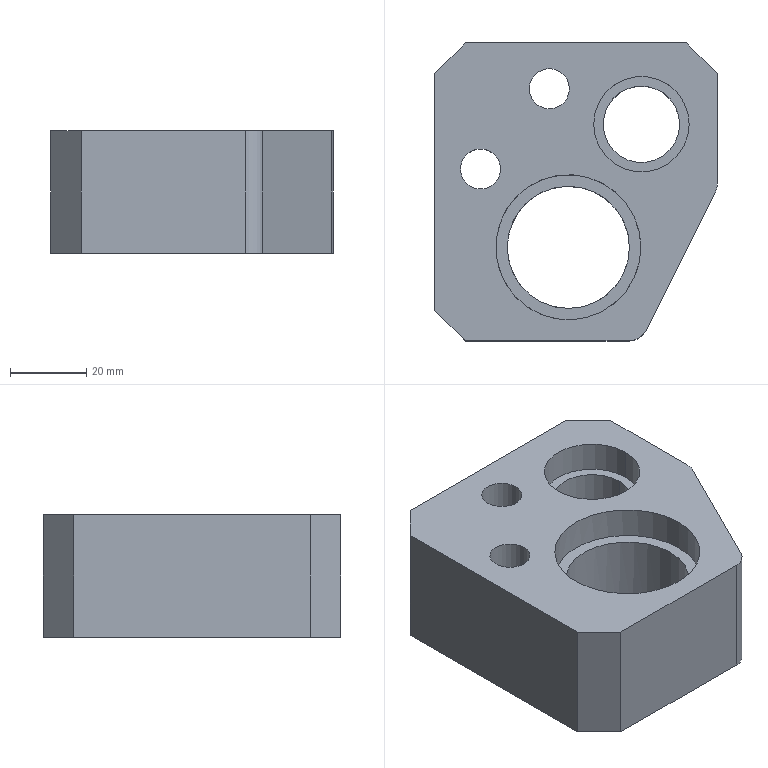Part | STEP file | lll_id3666_x_t | 1 solid | 26 faces | box 74 x 78 x 32 mm | volume 118554 mm3 | plane 14 | cylinder 12 | commonest cylinder face diameters 10 x2 10.5 x2 17 x2 20 x2 25 x2 32 x1
STEP:
#1=CARTESIAN_POINT('',(3317.117,63.788,77.5));
#2=VERTEX_POINT('',#1);
#3=CARTESIAN_POINT('',(3322.367,63.788,77.5));
#4=DIRECTION('',(0.,0.,1.));
#5=DIRECTION('',(-1.,0.,0.));
#6=AXIS2_PLACEMENT_3D('',#3,#4,#5);
#7=CIRCLE('',#6,5.25);
#8=EDGE_CURVE('',#2,#2,#7,.T.);
#9=ORIENTED_EDGE('',*,*,#8,.T.);
#10=EDGE_LOOP('',(#9));
#11=FACE_BOUND('',#10,.T.);
#12=CARTESIAN_POINT('',(3313.867,63.788,77.5));
#13=VERTEX_POINT('',#12);
#14=CARTESIAN_POINT('',(3322.367,63.788,77.5));
#15=DIRECTION('',(0.,0.,1.));
#16=DIRECTION('',(-1.,0.,0.));
#17=AXIS2_PLACEMENT_3D('',#14,#15,#16);
#18=CIRCLE('',#17,8.5);
#19=EDGE_CURVE('',#13,#13,#18,.T.);
#20=ORIENTED_EDGE('',*,*,#19,.F.);
#21=EDGE_LOOP('',(#20));
#22=FACE_BOUND('',#21,.T.);
#23=CARTESIAN_POINT('',(3322.367,63.788,77.5));
#24=DIRECTION('',(0.,0.,1.));
#25=DIRECTION('',(-1.,0.,0.));
#26=AXIS2_PLACEMENT_3D('',#23,#24,#25);
#27=PLANE('',#26);
#28=ADVANCED_FACE('',(#11,#22),#27,.F.);
#29=CARTESIAN_POINT('',(3326.367,43.288,84.3));
#30=VERTEX_POINT('',#29);
#31=CARTESIAN_POINT('',(3345.367,43.288,84.3));
#32=DIRECTION('',(0.,0.,1.));
#33=DIRECTION('',(-1.,0.,0.));
#34=AXIS2_PLACEMENT_3D('',#31,#32,#33);
#35=CIRCLE('',#34,19.);
#36=EDGE_CURVE('',#30,#30,#35,.T.);
#37=ORIENTED_EDGE('',*,*,#36,.T.);
#38=EDGE_LOOP('',(#37));
#39=FACE_BOUND('',#38,.T.);
#40=CARTESIAN_POINT('',(3329.367,43.288,84.3));
#41=VERTEX_POINT('',#40);
#42=CARTESIAN_POINT('',(3345.367,43.288,84.3));
#43=DIRECTION('',(0.,0.,1.));
#44=DIRECTION('',(-1.,0.,0.));
#45=AXIS2_PLACEMENT_3D('',#42,#43,#44);
#46=CIRCLE('',#45,16.);
#47=EDGE_CURVE('',#41,#41,#46,.T.);
#48=ORIENTED_EDGE('',*,*,#47,.F.);
#49=EDGE_LOOP('',(#48));
#50=FACE_BOUND('',#49,.T.);
#51=CARTESIAN_POINT('',(3345.367,52.038,84.3));
#52=DIRECTION('',(0.,0.,-1.));
#53=DIRECTION('',(0.,1.,0.));
#54=AXIS2_PLACEMENT_3D('',#51,#52,#53);
#55=PLANE('',#54);
#56=ADVANCED_FACE('',(#39,#50),#55,.F.);
#57=CARTESIAN_POINT('',(3352.,75.5,84.5));
#58=VERTEX_POINT('',#57);
#59=CARTESIAN_POINT('',(3377.,75.5,84.5));
#60=VERTEX_POINT('',#59);
#61=CARTESIAN_POINT('',(3364.5,75.5,84.5));
#62=DIRECTION('',(0.,0.,-1.));
#63=DIRECTION('',(1.,0.,0.));
#64=AXIS2_PLACEMENT_3D('',#61,#62,#63);
#65=CIRCLE('',#64,12.5);
#66=EDGE_CURVE('',#58,#60,#65,.T.);
#67=ORIENTED_EDGE('',*,*,#66,.F.);
#68=CARTESIAN_POINT('',(3364.5,75.5,84.5));
#69=DIRECTION('',(0.,0.,-1.));
#70=DIRECTION('',(1.,0.,0.));
#71=AXIS2_PLACEMENT_3D('',#68,#69,#70);
#72=CIRCLE('',#71,12.5);
#73=EDGE_CURVE('',#60,#58,#72,.T.);
#74=ORIENTED_EDGE('',*,*,#73,.F.);
#75=EDGE_LOOP('',(#67,#74));
#76=FACE_BOUND('',#75,.T.);
#77=CARTESIAN_POINT('',(3354.5,75.5,84.5));
#78=VERTEX_POINT('',#77);
#79=CARTESIAN_POINT('',(3374.5,75.5,84.5));
#80=VERTEX_POINT('',#79);
#81=CARTESIAN_POINT('',(3364.5,75.5,84.5));
#82=DIRECTION('',(0.,0.,-1.));
#83=DIRECTION('',(1.,0.,0.));
#84=AXIS2_PLACEMENT_3D('',#81,#82,#83);
#85=CIRCLE('',#84,10.);
#86=EDGE_CURVE('',#78,#80,#85,.T.);
#87=ORIENTED_EDGE('',*,*,#86,.T.);
#88=CARTESIAN_POINT('',(3364.5,75.5,84.5));
#89=DIRECTION('',(0.,0.,-1.));
#90=DIRECTION('',(1.,0.,0.));
#91=AXIS2_PLACEMENT_3D('',#88,#89,#90);
#92=CIRCLE('',#91,10.);
#93=EDGE_CURVE('',#80,#78,#92,.T.);
#94=ORIENTED_EDGE('',*,*,#93,.T.);
#95=EDGE_LOOP('',(#87,#94));
#96=FACE_BOUND('',#95,.T.);
#97=CARTESIAN_POINT('',(3375.75,75.5,84.5));
#98=DIRECTION('',(0.,0.,-1.));
#99=DIRECTION('',(1.,0.,0.));
#100=AXIS2_PLACEMENT_3D('',#97,#98,#99);
#101=PLANE('',#100);
#102=ADVANCED_FACE('',(#76,#96),#101,.F.);
#103=ORIENTED_EDGE('',*,*,#19,.T.);
#104=EDGE_LOOP('',(#103));
#105=FACE_BOUND('',#104,.T.);
#106=CARTESIAN_POINT('',(3313.867,63.788,60.5));
#107=VERTEX_POINT('',#106);
#108=CARTESIAN_POINT('',(3322.367,63.788,60.5));
#109=DIRECTION('',(0.,0.,-1.));
#110=DIRECTION('',(-1.,0.,0.));
#111=AXIS2_PLACEMENT_3D('',#108,#109,#110);
#112=CIRCLE('',#111,8.5);
#113=EDGE_CURVE('',#107,#107,#112,.T.);
#114=ORIENTED_EDGE('',*,*,#113,.T.);
#115=EDGE_LOOP('',(#114));
#116=FACE_BOUND('',#115,.T.);
#117=CARTESIAN_POINT('',(3322.367,63.788,60.5));
#118=DIRECTION('',(0.,0.,1.));
#119=DIRECTION('',(-1.,0.,0.));
#120=AXIS2_PLACEMENT_3D('',#117,#118,#119);
#121=CYLINDRICAL_SURFACE('',#120,8.5);
#122=ADVANCED_FACE('',(#105,#116),#121,.F.);
#123=CARTESIAN_POINT('',(3365.748,21.552,60.5));
#124=VERTEX_POINT('',#123);
#125=CARTESIAN_POINT('',(3361.276,18.788,60.5));
#126=VERTEX_POINT('',#125);
#127=CARTESIAN_POINT('',(3361.276,23.788,60.5));
#128=DIRECTION('',(0.,0.,-1.));
#129=DIRECTION('',(-1.,0.,0.));
#130=AXIS2_PLACEMENT_3D('',#127,#128,#129);
#131=CIRCLE('',#130,5.);
#132=EDGE_CURVE('',#124,#126,#131,.T.);
#133=ORIENTED_EDGE('',*,*,#132,.F.);
#134=CARTESIAN_POINT('',(3365.748,21.552,92.5));
#135=VERTEX_POINT('',#134);
#136=CARTESIAN_POINT('',(3365.748,21.552,-8.5));
#137=DIRECTION('',(0.,0.,-1.));
#138=VECTOR('',#137,1.);
#139=LINE('',#136,#138);
#140=EDGE_CURVE('',#135,#124,#139,.T.);
#141=ORIENTED_EDGE('',*,*,#140,.F.);
#142=CARTESIAN_POINT('',(3361.276,18.788,92.5));
#143=VERTEX_POINT('',#142);
#144=CARTESIAN_POINT('',(3361.276,23.788,92.5));
#145=DIRECTION('',(0.,0.,1.));
#146=DIRECTION('',(-1.,0.,0.));
#147=AXIS2_PLACEMENT_3D('',#144,#145,#146);
#148=CIRCLE('',#147,5.);
#149=EDGE_CURVE('',#143,#135,#148,.T.);
#150=ORIENTED_EDGE('',*,*,#149,.F.);
#151=CARTESIAN_POINT('',(3361.276,18.788,-8.5));
#152=DIRECTION('',(0.,0.,1.));
#153=VECTOR('',#152,1.);
#154=LINE('',#151,#153);
#155=EDGE_CURVE('',#126,#143,#154,.T.);
#156=ORIENTED_EDGE('',*,*,#155,.F.);
#157=EDGE_LOOP('',(#133,#141,#150,#156));
#158=FACE_OUTER_BOUND('',#157,.T.);
#159=CARTESIAN_POINT('',(3361.276,23.788,-8.5));
#160=DIRECTION('',(0.,0.,-1.));
#161=DIRECTION('',(1.,0.,0.));
#162=AXIS2_PLACEMENT_3D('',#159,#160,#161);
#163=CYLINDRICAL_SURFACE('',#162,5.);
#164=ADVANCED_FACE('',(#158),#163,.T.);
#165=CARTESIAN_POINT('',(3318.367,18.788,60.5));
#166=VERTEX_POINT('',#165);
#167=CARTESIAN_POINT('',(3282.176,18.788,60.5));
#168=DIRECTION('',(-1.,0.,0.));
#169=VECTOR('',#168,1.);
#170=LINE('',#167,#169);
#171=EDGE_CURVE('',#126,#166,#170,.T.);
#172=ORIENTED_EDGE('',*,*,#171,.F.);
#173=ORIENTED_EDGE('',*,*,#155,.T.);
#174=CARTESIAN_POINT('',(3318.367,18.788,92.5));
#175=VERTEX_POINT('',#174);
#176=CARTESIAN_POINT('',(3345.367,18.788,92.5));
#177=DIRECTION('',(1.,0.,0.));
#178=VECTOR('',#177,1.);
#179=LINE('',#176,#178);
#180=EDGE_CURVE('',#175,#143,#179,.T.);
#181=ORIENTED_EDGE('',*,*,#180,.F.);
#182=CARTESIAN_POINT('',(3318.367,18.788,-8.5));
#183=DIRECTION('',(0.,0.,-1.));
#184=VECTOR('',#183,1.);
#185=LINE('',#182,#184);
#186=EDGE_CURVE('',#175,#166,#185,.T.);
#187=ORIENTED_EDGE('',*,*,#186,.T.);
#188=EDGE_LOOP('',(#172,#173,#181,#187));
#189=FACE_OUTER_BOUND('',#188,.T.);
#190=CARTESIAN_POINT('',(3345.367,18.788,-8.5));
#191=DIRECTION('',(0.,-1.,0.));
#192=DIRECTION('',(0.,0.,-1.));
#193=AXIS2_PLACEMENT_3D('',#190,#191,#192);
#194=PLANE('',#193);
#195=ADVANCED_FACE('',(#189),#194,.T.);
#196=CARTESIAN_POINT('',(3310.367,26.788,60.5));
#197=VERTEX_POINT('',#196);
#198=CARTESIAN_POINT('',(3269.884,67.271,60.5));
#199=DIRECTION('',(-0.7071,0.7071,0.));
#200=VECTOR('',#199,1.);
#201=LINE('',#198,#200);
#202=EDGE_CURVE('',#166,#197,#201,.T.);
#203=ORIENTED_EDGE('',*,*,#202,.F.);
#204=ORIENTED_EDGE('',*,*,#186,.F.);
#205=CARTESIAN_POINT('',(3310.367,26.788,92.5));
#206=VERTEX_POINT('',#205);
#207=CARTESIAN_POINT('',(3264.934,72.22,92.5));
#208=DIRECTION('',(0.7071,-0.7071,0.));
#209=VECTOR('',#208,1.);
#210=LINE('',#207,#209);
#211=EDGE_CURVE('',#206,#175,#210,.T.);
#212=ORIENTED_EDGE('',*,*,#211,.F.);
#213=CARTESIAN_POINT('',(3310.367,26.788,-8.5));
#214=DIRECTION('',(0.,0.,1.));
#215=VECTOR('',#214,1.);
#216=LINE('',#213,#215);
#217=EDGE_CURVE('',#197,#206,#216,.T.);
#218=ORIENTED_EDGE('',*,*,#217,.F.);
#219=EDGE_LOOP('',(#203,#204,#212,#218));
#220=FACE_OUTER_BOUND('',#219,.T.);
#221=CARTESIAN_POINT('',(3310.367,26.788,-8.5));
#222=DIRECTION('',(0.7071,0.7071,0.));
#223=DIRECTION('',(0.,0.,1.));
#224=AXIS2_PLACEMENT_3D('',#221,#222,#223);
#225=PLANE('',#224);
#226=ADVANCED_FACE('',(#220),#225,.F.);
#227=CARTESIAN_POINT('',(3310.367,88.788,92.5));
#228=VERTEX_POINT('',#227);
#229=CARTESIAN_POINT('',(3310.367,74.513,92.5));
#230=DIRECTION('',(0.,-1.,0.));
#231=VECTOR('',#230,1.);
#232=LINE('',#229,#231);
#233=EDGE_CURVE('',#228,#206,#232,.T.);
#234=ORIENTED_EDGE('',*,*,#233,.F.);
#235=CARTESIAN_POINT('',(3310.367,88.788,60.5));
#236=VERTEX_POINT('',#235);
#237=CARTESIAN_POINT('',(3310.367,88.788,-8.5));
#238=DIRECTION('',(0.,0.,-1.));
#239=VECTOR('',#238,1.);
#240=LINE('',#237,#239);
#241=EDGE_CURVE('',#228,#236,#240,.T.);
#242=ORIENTED_EDGE('',*,*,#241,.T.);
#243=CARTESIAN_POINT('',(3310.367,69.563,60.5));
#244=DIRECTION('',(0.,1.,0.));
#245=VECTOR('',#244,1.);
#246=LINE('',#243,#245);
#247=EDGE_CURVE('',#197,#236,#246,.T.);
#248=ORIENTED_EDGE('',*,*,#247,.F.);
#249=ORIENTED_EDGE('',*,*,#217,.T.);
#250=EDGE_LOOP('',(#234,#242,#248,#249));
#251=FACE_OUTER_BOUND('',#250,.T.);
#252=CARTESIAN_POINT('',(3310.367,43.288,-8.5));
#253=DIRECTION('',(-1.,0.,0.));
#254=DIRECTION('',(0.,0.,-1.));
#255=AXIS2_PLACEMENT_3D('',#252,#253,#254);
#256=PLANE('',#255);
#257=ADVANCED_FACE('',(#251),#256,.T.);
#258=CARTESIAN_POINT('',(3318.367,96.788,60.5));
#259=VERTEX_POINT('',#258);
#260=CARTESIAN_POINT('',(3281.659,60.08,60.5));
#261=DIRECTION('',(0.7071,0.7071,0.));
#262=VECTOR('',#261,1.);
#263=LINE('',#260,#262);
#264=EDGE_CURVE('',#236,#259,#263,.T.);
#265=ORIENTED_EDGE('',*,*,#264,.F.);
#266=ORIENTED_EDGE('',*,*,#241,.F.);
#267=CARTESIAN_POINT('',(3318.367,96.788,92.5));
#268=VERTEX_POINT('',#267);
#269=CARTESIAN_POINT('',(3281.659,60.08,92.5));
#270=DIRECTION('',(-0.7071,-0.7071,0.));
#271=VECTOR('',#270,1.);
#272=LINE('',#269,#271);
#273=EDGE_CURVE('',#268,#228,#272,.T.);
#274=ORIENTED_EDGE('',*,*,#273,.F.);
#275=CARTESIAN_POINT('',(3318.367,96.788,-8.5));
#276=DIRECTION('',(0.,0.,1.));
#277=VECTOR('',#276,1.);
#278=LINE('',#275,#277);
#279=EDGE_CURVE('',#259,#268,#278,.T.);
#280=ORIENTED_EDGE('',*,*,#279,.F.);
#281=EDGE_LOOP('',(#265,#266,#274,#280));
#282=FACE_OUTER_BOUND('',#281,.T.);
#283=CARTESIAN_POINT('',(3318.367,96.788,-8.5));
#284=DIRECTION('',(0.7071,-0.7071,0.));
#285=DIRECTION('',(0.,0.,1.));
#286=AXIS2_PLACEMENT_3D('',#283,#284,#285);
#287=PLANE('',#286);
#288=ADVANCED_FACE('',(#282),#287,.F.);
#289=CARTESIAN_POINT('',(3376.366,96.788,92.5));
#290=VERTEX_POINT('',#289);
#291=CARTESIAN_POINT('',(3345.367,96.788,92.5));
#292=DIRECTION('',(-1.,0.,0.));
#293=VECTOR('',#292,1.);
#294=LINE('',#291,#293);
#295=EDGE_CURVE('',#290,#268,#294,.T.);
#296=ORIENTED_EDGE('',*,*,#295,.F.);
#297=CARTESIAN_POINT('',(3376.366,96.788,60.5));
#298=VERTEX_POINT('',#297);
#299=CARTESIAN_POINT('',(3376.366,96.788,-8.5));
#300=DIRECTION('',(0.,0.,-1.));
#301=VECTOR('',#300,1.);
#302=LINE('',#299,#301);
#303=EDGE_CURVE('',#290,#298,#302,.T.);
#304=ORIENTED_EDGE('',*,*,#303,.T.);
#305=CARTESIAN_POINT('',(3282.176,96.788,60.5));
#306=DIRECTION('',(1.,0.,0.));
#307=VECTOR('',#306,1.);
#308=LINE('',#305,#307);
#309=EDGE_CURVE('',#259,#298,#308,.T.);
#310=ORIENTED_EDGE('',*,*,#309,.F.);
#311=ORIENTED_EDGE('',*,*,#279,.T.);
#312=EDGE_LOOP('',(#296,#304,#310,#311));
#313=FACE_OUTER_BOUND('',#312,.T.);
#314=CARTESIAN_POINT('',(3345.367,96.788,-8.5));
#315=DIRECTION('',(0.,1.,0.));
#316=DIRECTION('',(0.,0.,1.));
#317=AXIS2_PLACEMENT_3D('',#314,#315,#316);
#318=PLANE('',#317);
#319=ADVANCED_FACE('',(#313),#318,.T.);
#320=CARTESIAN_POINT('',(3384.366,88.788,60.5));
#321=VERTEX_POINT('',#320);
#322=CARTESIAN_POINT('',(3342.383,130.771,60.5));
#323=DIRECTION('',(0.7071,-0.7071,0.));
#324=VECTOR('',#323,1.);
#325=LINE('',#322,#324);
#326=EDGE_CURVE('',#298,#321,#325,.T.);
#327=ORIENTED_EDGE('',*,*,#326,.F.);
#328=ORIENTED_EDGE('',*,*,#303,.F.);
#329=CARTESIAN_POINT('',(3384.366,88.788,92.5));
#330=VERTEX_POINT('',#329);
#331=CARTESIAN_POINT('',(3337.434,135.72,92.5));
#332=DIRECTION('',(-0.7071,0.7071,0.));
#333=VECTOR('',#332,1.);
#334=LINE('',#331,#333);
#335=EDGE_CURVE('',#330,#290,#334,.T.);
#336=ORIENTED_EDGE('',*,*,#335,.F.);
#337=CARTESIAN_POINT('',(3384.366,88.788,-8.5));
#338=DIRECTION('',(0.,0.,1.));
#339=VECTOR('',#338,1.);
#340=LINE('',#337,#339);
#341=EDGE_CURVE('',#321,#330,#340,.T.);
#342=ORIENTED_EDGE('',*,*,#341,.F.);
#343=EDGE_LOOP('',(#327,#328,#336,#342));
#344=FACE_OUTER_BOUND('',#343,.T.);
#345=CARTESIAN_POINT('',(3384.366,88.788,-8.5));
#346=DIRECTION('',(-0.7071,-0.7071,0.));
#347=DIRECTION('',(0.,0.,1.));
#348=AXIS2_PLACEMENT_3D('',#345,#346,#347);
#349=PLANE('',#348);
#350=ADVANCED_FACE('',(#344),#349,.F.);
#351=CARTESIAN_POINT('',(3384.366,59.968,92.5));
#352=VERTEX_POINT('',#351);
#353=CARTESIAN_POINT('',(3384.366,69.563,92.5));
#354=DIRECTION('',(0.,1.,0.));
#355=VECTOR('',#354,1.);
#356=LINE('',#353,#355);
#357=EDGE_CURVE('',#352,#330,#356,.T.);
#358=ORIENTED_EDGE('',*,*,#357,.F.);
#359=CARTESIAN_POINT('',(3384.366,59.968,60.5));
#360=VERTEX_POINT('',#359);
#361=CARTESIAN_POINT('',(3384.366,59.968,-8.5));
#362=DIRECTION('',(0.,0.,-1.));
#363=VECTOR('',#362,1.);
#364=LINE('',#361,#363);
#365=EDGE_CURVE('',#352,#360,#364,.T.);
#366=ORIENTED_EDGE('',*,*,#365,.T.);
#367=CARTESIAN_POINT('',(3384.366,69.563,60.5));
#368=DIRECTION('',(0.,-1.,0.));
#369=VECTOR('',#368,1.);
#370=LINE('',#367,#369);
#371=EDGE_CURVE('',#321,#360,#370,.T.);
#372=ORIENTED_EDGE('',*,*,#371,.F.);
#373=ORIENTED_EDGE('',*,*,#341,.T.);
#374=EDGE_LOOP('',(#358,#366,#372,#373));
#375=FACE_OUTER_BOUND('',#374,.T.);
#376=CARTESIAN_POINT('',(3384.366,38.338,-8.5));
#377=DIRECTION('',(1.,0.,0.));
#378=DIRECTION('',(0.,0.,1.));
#379=AXIS2_PLACEMENT_3D('',#376,#377,#378);
#380=PLANE('',#379);
#381=ADVANCED_FACE('',(#375),#380,.T.);
#382=CARTESIAN_POINT('',(3383.838,57.732,92.5));
#383=VERTEX_POINT('',#382);
#384=CARTESIAN_POINT('',(3379.366,59.968,92.5));
#385=DIRECTION('',(0.,0.,1.));
#386=DIRECTION('',(-1.,0.,0.));
#387=AXIS2_PLACEMENT_3D('',#384,#385,#386);
#388=CIRCLE('',#387,5.);
#389=EDGE_CURVE('',#383,#352,#388,.T.);
#390=ORIENTED_EDGE('',*,*,#389,.F.);
#391=CARTESIAN_POINT('',(3383.838,57.732,60.5));
#392=VERTEX_POINT('',#391);
#393=CARTESIAN_POINT('',(3383.838,57.732,-8.5));
#394=DIRECTION('',(0.,0.,1.));
#395=VECTOR('',#394,1.);
#396=LINE('',#393,#395);
#397=EDGE_CURVE('',#392,#383,#396,.T.);
#398=ORIENTED_EDGE('',*,*,#397,.F.);
#399=CARTESIAN_POINT('',(3379.366,59.968,60.5));
#400=DIRECTION('',(0.,0.,-1.));
#401=DIRECTION('',(-1.,0.,0.));
#402=AXIS2_PLACEMENT_3D('',#399,#400,#401);
#403=CIRCLE('',#402,5.);
#404=EDGE_CURVE('',#360,#392,#403,.T.);
#405=ORIENTED_EDGE('',*,*,#404,.F.);
#406=ORIENTED_EDGE('',*,*,#365,.F.);
#407=EDGE_LOOP('',(#390,#398,#405,#406));
#408=FACE_OUTER_BOUND('',#407,.T.);
#409=CARTESIAN_POINT('',(3379.366,59.968,-8.5));
#410=DIRECTION('',(0.,0.,1.));
#411=DIRECTION('',(-1.,0.,0.));
#412=AXIS2_PLACEMENT_3D('',#409,#410,#411);
#413=CYLINDRICAL_SURFACE('',#412,5.);
#414=ADVANCED_FACE('',(#408),#413,.T.);
#415=CARTESIAN_POINT('',(3368.239,26.532,60.5));
#416=DIRECTION('',(-0.4472,-0.8944,0.));
#417=VECTOR('',#416,1.);
#418=LINE('',#415,#417);
#419=EDGE_CURVE('',#392,#124,#418,.T.);
#420=ORIENTED_EDGE('',*,*,#419,.F.);
#421=ORIENTED_EDGE('',*,*,#397,.T.);
#422=CARTESIAN_POINT('',(3369.229,28.512,92.5));
#423=DIRECTION('',(0.4472,0.8944,0.));
#424=VECTOR('',#423,1.);
#425=LINE('',#422,#424);
#426=EDGE_CURVE('',#135,#383,#425,.T.);
#427=ORIENTED_EDGE('',*,*,#426,.F.);
#428=ORIENTED_EDGE('',*,*,#140,.T.);
#429=EDGE_LOOP('',(#420,#421,#427,#428));
#430=FACE_OUTER_BOUND('',#429,.T.);
#431=CARTESIAN_POINT('',(3384.566,59.188,-8.5));
#432=DIRECTION('',(-0.8944,0.4472,0.));
#433=DIRECTION('',(0.,0.,-1.));
#434=AXIS2_PLACEMENT_3D('',#431,#432,#433);
#435=PLANE('',#434);
#436=ADVANCED_FACE('',(#430),#435,.F.);
#437=CARTESIAN_POINT('',(3317.117,63.788,92.5));
#438=VERTEX_POINT('',#437);
#439=CARTESIAN_POINT('',(3322.367,63.788,92.5));
#440=DIRECTION('',(0.,0.,-1.));
#441=DIRECTION('',(-1.,0.,0.));
#442=AXIS2_PLACEMENT_3D('',#439,#440,#441);
#443=CIRCLE('',#442,5.25);
#444=EDGE_CURVE('',#438,#438,#443,.T.);
#445=ORIENTED_EDGE('',*,*,#444,.F.);
#446=EDGE_LOOP('',(#445));
#447=FACE_BOUND('',#446,.T.);
#448=ORIENTED_EDGE('',*,*,#8,.F.);
#449=EDGE_LOOP('',(#448));
#450=FACE_BOUND('',#449,.T.);
#451=CARTESIAN_POINT('',(3322.367,63.788,160.5));
#452=DIRECTION('',(0.,0.,1.));
#453=DIRECTION('',(-1.,0.,0.));
#454=AXIS2_PLACEMENT_3D('',#451,#452,#453);
#455=CYLINDRICAL_SURFACE('',#454,5.25);
#456=ADVANCED_FACE('',(#447,#450),#455,.F.);
#457=CARTESIAN_POINT('',(3364.367,43.288,92.5));
#458=VERTEX_POINT('',#457);
#459=CARTESIAN_POINT('',(3345.367,43.288,92.5));
#460=DIRECTION('',(0.,0.,-1.));
#461=DIRECTION('',(1.,0.,0.));
#462=AXIS2_PLACEMENT_3D('',#459,#460,#461);
#463=CIRCLE('',#462,19.);
#464=EDGE_CURVE('',#458,#458,#463,.T.);
#465=ORIENTED_EDGE('',*,*,#464,.F.);
#466=EDGE_LOOP('',(#465));
#467=FACE_BOUND('',#466,.T.);
#468=ORIENTED_EDGE('',*,*,#36,.F.);
#469=EDGE_LOOP('',(#468));
#470=FACE_BOUND('',#469,.T.);
#471=CARTESIAN_POINT('',(3345.367,43.288,90.));
#472=DIRECTION('',(0.,0.,-1.));
#473=DIRECTION('',(0.,-1.,0.));
#474=AXIS2_PLACEMENT_3D('',#471,#472,#473);
#475=CYLINDRICAL_SURFACE('',#474,19.);
#476=ADVANCED_FACE('',(#467,#470),#475,.F.);
#477=CARTESIAN_POINT('',(3377.,75.5,92.5));
#478=VERTEX_POINT('',#477);
#479=CARTESIAN_POINT('',(3377.,75.5,88.5));
#480=DIRECTION('',(0.,0.,-1.));
#481=VECTOR('',#480,1.);
#482=LINE('',#479,#481);
#483=EDGE_CURVE('',#478,#60,#482,.T.);
#484=ORIENTED_EDGE('',*,*,#483,.T.);
#485=ORIENTED_EDGE('',*,*,#73,.T.);
#486=CARTESIAN_POINT('',(3352.,75.5,92.5));
#487=VERTEX_POINT('',#486);
#488=CARTESIAN_POINT('',(3352.,75.5,88.5));
#489=DIRECTION('',(0.,0.,1.));
#490=VECTOR('',#489,1.);
#491=LINE('',#488,#490);
#492=EDGE_CURVE('',#58,#487,#491,.T.);
#493=ORIENTED_EDGE('',*,*,#492,.T.);
#494=CARTESIAN_POINT('',(3364.5,75.5,92.5));
#495=DIRECTION('',(0.,0.,1.));
#496=DIRECTION('',(1.,0.,0.));
#497=AXIS2_PLACEMENT_3D('',#494,#495,#496);
#498=CIRCLE('',#497,12.5);
#499=EDGE_CURVE('',#487,#478,#498,.T.);
#500=ORIENTED_EDGE('',*,*,#499,.T.);
#501=EDGE_LOOP('',(#484,#485,#493,#500));
#502=FACE_OUTER_BOUND('',#501,.T.);
#503=CARTESIAN_POINT('',(3364.5,75.5,88.5));
#504=DIRECTION('',(0.,0.,-1.));
#505=DIRECTION('',(-1.,0.,0.));
#506=AXIS2_PLACEMENT_3D('',#503,#504,#505);
#507=CYLINDRICAL_SURFACE('',#506,12.5);
#508=ADVANCED_FACE('',(#502),#507,.F.);
#509=ORIENTED_EDGE('',*,*,#483,.F.);
#510=CARTESIAN_POINT('',(3364.5,75.5,92.5));
#511=DIRECTION('',(0.,0.,1.));
#512=DIRECTION('',(1.,0.,0.));
#513=AXIS2_PLACEMENT_3D('',#510,#511,#512);
#514=CIRCLE('',#513,12.5);
#515=EDGE_CURVE('',#478,#487,#514,.T.);
#516=ORIENTED_EDGE('',*,*,#515,.T.);
#517=ORIENTED_EDGE('',*,*,#492,.F.);
#518=ORIENTED_EDGE('',*,*,#66,.T.);
#519=EDGE_LOOP('',(#509,#516,#517,#518));
#520=FACE_OUTER_BOUND('',#519,.T.);
#521=CARTESIAN_POINT('',(3364.5,75.5,88.5));
#522=DIRECTION('',(0.,0.,-1.));
#523=DIRECTION('',(-1.,0.,0.));
#524=AXIS2_PLACEMENT_3D('',#521,#522,#523);
#525=CYLINDRICAL_SURFACE('',#524,12.5);
#526=ADVANCED_FACE('',(#520),#525,.F.);
#527=CARTESIAN_POINT('',(3345.617,84.788,92.5));
#528=VERTEX_POINT('',#527);
#529=CARTESIAN_POINT('',(3340.367,84.788,92.5));
#530=DIRECTION('',(0.,0.,1.));
#531=DIRECTION('',(1.,0.,0.));
#532=AXIS2_PLACEMENT_3D('',#529,#530,#531);
#533=CIRCLE('',#532,5.25);
#534=EDGE_CURVE('',#528,#528,#533,.T.);
#535=ORIENTED_EDGE('',*,*,#534,.F.);
#536=EDGE_LOOP('',(#535));
#537=FACE_BOUND('',#536,.T.);
#538=ORIENTED_EDGE('',*,*,#515,.F.);
#539=ORIENTED_EDGE('',*,*,#499,.F.);
#540=EDGE_LOOP('',(#538,#539));
#541=FACE_BOUND('',#540,.T.);
#542=ORIENTED_EDGE('',*,*,#464,.T.);
#543=EDGE_LOOP('',(#542));
#544=FACE_BOUND('',#543,.T.);
#545=ORIENTED_EDGE('',*,*,#444,.T.);
#546=EDGE_LOOP('',(#545));
#547=FACE_BOUND('',#546,.T.);
#548=ORIENTED_EDGE('',*,*,#426,.T.);
#549=ORIENTED_EDGE('',*,*,#389,.T.);
#550=ORIENTED_EDGE('',*,*,#357,.T.);
#551=ORIENTED_EDGE('',*,*,#335,.T.);
#552=ORIENTED_EDGE('',*,*,#295,.T.);
#553=ORIENTED_EDGE('',*,*,#273,.T.);
#554=ORIENTED_EDGE('',*,*,#233,.T.);
#555=ORIENTED_EDGE('',*,*,#211,.T.);
#556=ORIENTED_EDGE('',*,*,#180,.T.);
#557=ORIENTED_EDGE('',*,*,#149,.T.);
#558=EDGE_LOOP('',(#548,#549,#550,#551,#552,#553,#554,#555,#556,#557));
#559=FACE_BOUND('',#558,.T.);
#560=CARTESIAN_POINT('',(3277.227,74.513,92.5));
#561=DIRECTION('',(0.,0.,1.));
#562=DIRECTION('',(-1.,0.,0.));
#563=AXIS2_PLACEMENT_3D('',#560,#561,#562);
#564=PLANE('',#563);
#565=ADVANCED_FACE('',(#537,#541,#544,#547,#559),#564,.T.);
#566=CARTESIAN_POINT('',(3361.367,43.288,60.5));
#567=VERTEX_POINT('',#566);
#568=CARTESIAN_POINT('',(3345.367,43.288,60.5));
#569=DIRECTION('',(0.,0.,1.));
#570=DIRECTION('',(1.,0.,0.));
#571=AXIS2_PLACEMENT_3D('',#568,#569,#570);
#572=CIRCLE('',#571,16.);
#573=EDGE_CURVE('',#567,#567,#572,.T.);
#574=ORIENTED_EDGE('',*,*,#573,.F.);
#575=EDGE_LOOP('',(#574));
#576=FACE_BOUND('',#575,.T.);
#577=ORIENTED_EDGE('',*,*,#47,.T.);
#578=EDGE_LOOP('',(#577));
#579=FACE_BOUND('',#578,.T.);
#580=CARTESIAN_POINT('',(3345.367,43.288,44.8));
#581=DIRECTION('',(0.,0.,-1.));
#582=DIRECTION('',(0.,-1.,0.));
#583=AXIS2_PLACEMENT_3D('',#580,#581,#582);
#584=CYLINDRICAL_SURFACE('',#583,16.);
#585=ADVANCED_FACE('',(#576,#579),#584,.F.);
#586=CARTESIAN_POINT('',(3374.5,75.5,60.5));
#587=VERTEX_POINT('',#586);
#588=CARTESIAN_POINT('',(3354.5,75.5,60.5));
#589=VERTEX_POINT('',#588);
#590=CARTESIAN_POINT('',(3364.5,75.5,60.5));
#591=DIRECTION('',(0.,0.,-1.));
#592=DIRECTION('',(-1.,0.,0.));
#593=AXIS2_PLACEMENT_3D('',#590,#591,#592);
#594=CIRCLE('',#593,10.);
#595=EDGE_CURVE('',#587,#589,#594,.T.);
#596=ORIENTED_EDGE('',*,*,#595,.T.);
#597=CARTESIAN_POINT('',(3354.5,75.5,38.5));
#598=DIRECTION('',(0.,0.,1.));
#599=VECTOR('',#598,1.);
#600=LINE('',#597,#599);
#601=EDGE_CURVE('',#589,#78,#600,.T.);
#602=ORIENTED_EDGE('',*,*,#601,.T.);
#603=ORIENTED_EDGE('',*,*,#93,.F.);
#604=CARTESIAN_POINT('',(3374.5,75.5,38.5));
#605=DIRECTION('',(0.,0.,-1.));
#606=VECTOR('',#605,1.);
#607=LINE('',#604,#606);
#608=EDGE_CURVE('',#80,#587,#607,.T.);
#609=ORIENTED_EDGE('',*,*,#608,.T.);
#610=EDGE_LOOP('',(#596,#602,#603,#609));
#611=FACE_OUTER_BOUND('',#610,.T.);
#612=CARTESIAN_POINT('',(3364.5,75.5,38.5));
#613=DIRECTION('',(0.,0.,-1.));
#614=DIRECTION('',(-1.,0.,0.));
#615=AXIS2_PLACEMENT_3D('',#612,#613,#614);
#616=CYLINDRICAL_SURFACE('',#615,10.);
#617=ADVANCED_FACE('',(#611),#616,.F.);
#618=CARTESIAN_POINT('',(3364.5,75.5,60.5));
#619=DIRECTION('',(0.,0.,-1.));
#620=DIRECTION('',(-1.,0.,0.));
#621=AXIS2_PLACEMENT_3D('',#618,#619,#620);
#622=CIRCLE('',#621,10.);
#623=EDGE_CURVE('',#589,#587,#622,.T.);
#624=ORIENTED_EDGE('',*,*,#623,.T.);
#625=ORIENTED_EDGE('',*,*,#608,.F.);
#626=ORIENTED_EDGE('',*,*,#86,.F.);
#627=ORIENTED_EDGE('',*,*,#601,.F.);
#628=EDGE_LOOP('',(#624,#625,#626,#627));
#629=FACE_OUTER_BOUND('',#628,.T.);
#630=CARTESIAN_POINT('',(3364.5,75.5,38.5));
#631=DIRECTION('',(0.,0.,-1.));
#632=DIRECTION('',(-1.,0.,0.));
#633=AXIS2_PLACEMENT_3D('',#630,#631,#632);
#634=CYLINDRICAL_SURFACE('',#633,10.);
#635=ADVANCED_FACE('',(#629),#634,.F.);
#636=CARTESIAN_POINT('',(3348.867,84.788,60.5));
#637=VERTEX_POINT('',#636);
#638=CARTESIAN_POINT('',(3340.367,84.788,60.5));
#639=DIRECTION('',(0.,0.,-1.));
#640=DIRECTION('',(1.,0.,0.));
#641=AXIS2_PLACEMENT_3D('',#638,#639,#640);
#642=CIRCLE('',#641,8.5);
#643=EDGE_CURVE('',#637,#637,#642,.T.);
#644=ORIENTED_EDGE('',*,*,#643,.F.);
#645=EDGE_LOOP('',(#644));
#646=FACE_BOUND('',#645,.T.);
#647=ORIENTED_EDGE('',*,*,#623,.F.);
#648=ORIENTED_EDGE('',*,*,#595,.F.);
#649=EDGE_LOOP('',(#647,#648));
#650=FACE_BOUND('',#649,.T.);
#651=ORIENTED_EDGE('',*,*,#573,.T.);
#652=EDGE_LOOP('',(#651));
#653=FACE_BOUND('',#652,.T.);
#654=ORIENTED_EDGE('',*,*,#371,.T.);
#655=ORIENTED_EDGE('',*,*,#404,.T.);
#656=ORIENTED_EDGE('',*,*,#419,.T.);
#657=ORIENTED_EDGE('',*,*,#132,.T.);
#658=ORIENTED_EDGE('',*,*,#171,.T.);
#659=ORIENTED_EDGE('',*,*,#202,.T.);
#660=ORIENTED_EDGE('',*,*,#247,.T.);
#661=ORIENTED_EDGE('',*,*,#264,.T.);
#662=ORIENTED_EDGE('',*,*,#309,.T.);
#663=ORIENTED_EDGE('',*,*,#326,.T.);
#664=EDGE_LOOP('',(#654,#655,#656,#657,#658,#659,#660,#661,#662,#663));
#665=FACE_BOUND('',#664,.T.);
#666=ORIENTED_EDGE('',*,*,#113,.F.);
#667=EDGE_LOOP('',(#666));
#668=FACE_BOUND('',#667,.T.);
#669=CARTESIAN_POINT('',(3282.176,69.563,60.5));
#670=DIRECTION('',(0.,0.,1.));
#671=DIRECTION('',(-1.,0.,0.));
#672=AXIS2_PLACEMENT_3D('',#669,#670,#671);
#673=PLANE('',#672);
#674=ADVANCED_FACE('',(#646,#650,#653,#665,#668),#673,.F.);
#675=CARTESIAN_POINT('',(3335.117,84.788,77.5));
#676=VERTEX_POINT('',#675);
#677=CARTESIAN_POINT('',(3340.367,84.788,77.5));
#678=DIRECTION('',(0.,0.,1.));
#679=DIRECTION('',(-1.,0.,0.));
#680=AXIS2_PLACEMENT_3D('',#677,#678,#679);
#681=CIRCLE('',#680,5.25);
#682=EDGE_CURVE('',#676,#676,#681,.T.);
#683=ORIENTED_EDGE('',*,*,#682,.T.);
#684=EDGE_LOOP('',(#683));
#685=FACE_BOUND('',#684,.T.);
#686=CARTESIAN_POINT('',(3331.867,84.788,77.5));
#687=VERTEX_POINT('',#686);
#688=CARTESIAN_POINT('',(3340.367,84.788,77.5));
#689=DIRECTION('',(0.,0.,1.));
#690=DIRECTION('',(-1.,0.,0.));
#691=AXIS2_PLACEMENT_3D('',#688,#689,#690);
#692=CIRCLE('',#691,8.5);
#693=EDGE_CURVE('',#687,#687,#692,.T.);
#694=ORIENTED_EDGE('',*,*,#693,.F.);
#695=EDGE_LOOP('',(#694));
#696=FACE_BOUND('',#695,.T.);
#697=CARTESIAN_POINT('',(3340.367,84.788,77.5));
#698=DIRECTION('',(0.,0.,1.));
#699=DIRECTION('',(-1.,0.,0.));
#700=AXIS2_PLACEMENT_3D('',#697,#698,#699);
#701=PLANE('',#700);
#702=ADVANCED_FACE('',(#685,#696),#701,.F.);
#703=ORIENTED_EDGE('',*,*,#534,.T.);
#704=EDGE_LOOP('',(#703));
#705=FACE_BOUND('',#704,.T.);
#706=ORIENTED_EDGE('',*,*,#682,.F.);
#707=EDGE_LOOP('',(#706));
#708=FACE_BOUND('',#707,.T.);
#709=CARTESIAN_POINT('',(3340.367,84.788,160.5));
#710=DIRECTION('',(0.,0.,1.));
#711=DIRECTION('',(-1.,0.,0.));
#712=AXIS2_PLACEMENT_3D('',#709,#710,#711);
#713=CYLINDRICAL_SURFACE('',#712,5.25);
#714=ADVANCED_FACE('',(#705,#708),#713,.F.);
#715=ORIENTED_EDGE('',*,*,#693,.T.);
#716=EDGE_LOOP('',(#715));
#717=FACE_BOUND('',#716,.T.);
#718=ORIENTED_EDGE('',*,*,#643,.T.);
#719=EDGE_LOOP('',(#718));
#720=FACE_BOUND('',#719,.T.);
#721=CARTESIAN_POINT('',(3340.367,84.788,60.5));
#722=DIRECTION('',(0.,0.,1.));
#723=DIRECTION('',(-1.,0.,0.));
#724=AXIS2_PLACEMENT_3D('',#721,#722,#723);
#725=CYLINDRICAL_SURFACE('',#724,8.5);
#726=ADVANCED_FACE('',(#717,#720),#725,.F.);
#727=CLOSED_SHELL('',(#28,#56,#102,#122,#164,#195,#226,#257,#288,#319,#350,#381,#414,#436,#456,#476,#508,#526,#565,#585,#617,#635,#674,#702,#714,#726));
#728=MANIFOLD_SOLID_BREP('',#727);
#729=(LENGTH_UNIT()NAMED_UNIT(*)SI_UNIT(.MILLI.,.METRE.));
#730=UNCERTAINTY_MEASURE_WITH_UNIT(LENGTH_MEASURE(0.00002),#729,'','');
#731=(NAMED_UNIT(*)PLANE_ANGLE_UNIT()SI_UNIT($,.RADIAN.));
#732=PLANE_ANGLE_MEASURE_WITH_UNIT(PLANE_ANGLE_MEASURE(0.01745),#731);
#733=DIMENSIONAL_EXPONENTS(0.,0.,0.,0.,0.,0.,0.);
#734=(CONVERSION_BASED_UNIT('DEGREE',#732)NAMED_UNIT(#733)PLANE_ANGLE_UNIT());
#735=(NAMED_UNIT(*)SI_UNIT($,.STERADIAN.)SOLID_ANGLE_UNIT());
#736=(GEOMETRIC_REPRESENTATION_CONTEXT(3)GLOBAL_UNCERTAINTY_ASSIGNED_CONTEXT((#730))GLOBAL_UNIT_ASSIGNED_CONTEXT((#729,#734,#735))REPRESENTATION_CONTEXT('',''));
#737=ADVANCED_BREP_SHAPE_REPRESENTATION('',(#728),#736);